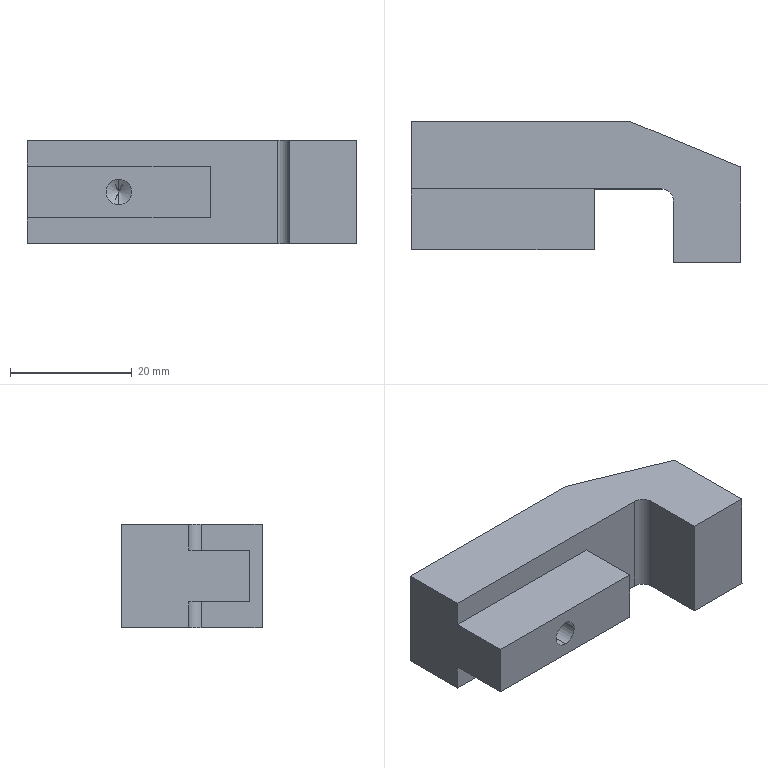Part | STEP file | PN_0002  Clamp_Default | 1 solid | 18 faces | box 54 x 23 x 17 mm | volume 13573 mm3 | plane 13 | cylinder 3 | cone 2 | commonest cylinder face diameters 4.2 x2 4 x1
STEP:
#1=CARTESIAN_POINT('',(0.,0.,0.));
#2=DIRECTION('',(0.,0.,1.));
#3=DIRECTION('',(1.,0.,0.));
#4=AXIS2_PLACEMENT_3D('',#1,#2,#3);
#5=CARTESIAN_POINT('',(15.,-7.,-2.1));
#6=VERTEX_POINT('',#5);
#7=CARTESIAN_POINT('',(15.,-21.,-2.1));
#8=VERTEX_POINT('',#7);
#9=CARTESIAN_POINT('',(15.,-21.,-2.1));
#10=DIRECTION('',(0.,-1.,0.));
#11=VECTOR('',#10,1.);
#12=LINE('',#9,#11);
#13=CARTESIAN_POINT('',(15.,-21.,0.));
#14=DIRECTION('',(0.,-1.,0.));
#15=DIRECTION('',(0.,0.,-1.));
#16=AXIS2_PLACEMENT_3D('',#13,#14,#15);
#17=CYLINDRICAL_SURFACE('',#16,2.1);
#18=CARTESIAN_POINT('',(6.283,0.));
#19=DIRECTION('',(0.,1.));
#20=VECTOR('',#19,1.);
#21=LINE('',#18,#20);
#22=(GEOMETRIC_REPRESENTATION_CONTEXT(2)PARAMETRIC_REPRESENTATION_CONTEXT()REPRESENTATION_CONTEXT('',''));
#23=DEFINITIONAL_REPRESENTATION('',(#21),#22);
#24=PCURVE('',#17,#23);
#25=CARTESIAN_POINT('',(15.,-21.,0.));
#26=DIRECTION('',(0.,-1.,0.));
#27=DIRECTION('',(0.,0.,-1.));
#28=AXIS2_PLACEMENT_3D('',#25,#26,#27);
#29=CYLINDRICAL_SURFACE('',#28,2.1);
#30=CARTESIAN_POINT('',(0.,0.));
#31=DIRECTION('',(0.,1.));
#32=VECTOR('',#31,1.);
#33=LINE('',#30,#32);
#34=(GEOMETRIC_REPRESENTATION_CONTEXT(2)PARAMETRIC_REPRESENTATION_CONTEXT()REPRESENTATION_CONTEXT('',''));
#35=DEFINITIONAL_REPRESENTATION('',(#33),#34);
#36=PCURVE('',#29,#35);
#37=SURFACE_CURVE('',#12,(#24,#36),.PCURVE_S1.);
#38=EDGE_CURVE('',#6,#8,#37,.T.);
#39=ORIENTED_EDGE('',*,*,#38,.T.);
#40=CARTESIAN_POINT('',(15.,-21.,2.1));
#41=VERTEX_POINT('',#40);
#42=CARTESIAN_POINT('',(15.,-21.,0.));
#43=DIRECTION('',(0.,-1.,0.));
#44=DIRECTION('',(0.,0.,-1.));
#45=AXIS2_PLACEMENT_3D('',#42,#43,#44);
#46=CIRCLE('',#45,2.1);
#47=CARTESIAN_POINT('',(0.,0.));
#48=DIRECTION('',(1.,0.));
#49=VECTOR('',#48,1.);
#50=LINE('',#47,#49);
#51=(GEOMETRIC_REPRESENTATION_CONTEXT(2)PARAMETRIC_REPRESENTATION_CONTEXT()REPRESENTATION_CONTEXT('',''));
#52=DEFINITIONAL_REPRESENTATION('',(#50),#51);
#53=PCURVE('',#17,#52);
#54=CARTESIAN_POINT('',(0.,-21.,0.));
#55=DIRECTION('',(0.,-1.,0.));
#56=DIRECTION('',(1.,0.,0.));
#57=AXIS2_PLACEMENT_3D('',#54,#55,#56);
#58=PLANE('',#57);
#59=CARTESIAN_POINT('',(15.,0.));
#60=DIRECTION('',(0.,-1.));
#61=AXIS2_PLACEMENT_2D('',#59,#60);
#62=CIRCLE('',#61,2.1);
#63=(GEOMETRIC_REPRESENTATION_CONTEXT(2)PARAMETRIC_REPRESENTATION_CONTEXT()REPRESENTATION_CONTEXT('',''));
#64=DEFINITIONAL_REPRESENTATION('',(#62),#63);
#65=PCURVE('',#58,#64);
#66=SURFACE_CURVE('',#46,(#53,#65),.PCURVE_S1.);
#67=EDGE_CURVE('',#41,#8,#66,.T.);
#68=ORIENTED_EDGE('',*,*,#67,.F.);
#69=CARTESIAN_POINT('',(15.,-7.,2.1));
#70=VERTEX_POINT('',#69);
#71=CARTESIAN_POINT('',(15.,-21.,2.1));
#72=DIRECTION('',(0.,-1.,0.));
#73=VECTOR('',#72,1.);
#74=LINE('',#71,#73);
#75=CARTESIAN_POINT('',(3.142,0.));
#76=DIRECTION('',(0.,1.));
#77=VECTOR('',#76,1.);
#78=LINE('',#75,#77);
#79=(GEOMETRIC_REPRESENTATION_CONTEXT(2)PARAMETRIC_REPRESENTATION_CONTEXT()REPRESENTATION_CONTEXT('',''));
#80=DEFINITIONAL_REPRESENTATION('',(#78),#79);
#81=PCURVE('',#17,#80);
#82=CARTESIAN_POINT('',(3.142,0.));
#83=DIRECTION('',(0.,1.));
#84=VECTOR('',#83,1.);
#85=LINE('',#82,#84);
#86=(GEOMETRIC_REPRESENTATION_CONTEXT(2)PARAMETRIC_REPRESENTATION_CONTEXT()REPRESENTATION_CONTEXT('',''));
#87=DEFINITIONAL_REPRESENTATION('',(#85),#86);
#88=PCURVE('',#29,#87);
#89=SURFACE_CURVE('',#74,(#81,#88),.PCURVE_S1.);
#90=EDGE_CURVE('',#70,#41,#89,.T.);
#91=ORIENTED_EDGE('',*,*,#90,.F.);
#92=CARTESIAN_POINT('',(15.,-7.,0.));
#93=DIRECTION('',(0.,-1.,0.));
#94=DIRECTION('',(0.,0.,-1.));
#95=AXIS2_PLACEMENT_3D('',#92,#93,#94);
#96=CIRCLE('',#95,2.1);
#97=CARTESIAN_POINT('',(0.,-14.));
#98=DIRECTION('',(1.,0.));
#99=VECTOR('',#98,1.);
#100=LINE('',#97,#99);
#101=(GEOMETRIC_REPRESENTATION_CONTEXT(2)PARAMETRIC_REPRESENTATION_CONTEXT()REPRESENTATION_CONTEXT('',''));
#102=DEFINITIONAL_REPRESENTATION('',(#100),#101);
#103=PCURVE('',#17,#102);
#104=CARTESIAN_POINT('',(15.,-7.,0.));
#105=DIRECTION('',(0.,-1.,0.));
#106=DIRECTION('',(0.,0.,-1.));
#107=AXIS2_PLACEMENT_3D('',#104,#105,#106);
#108=CONICAL_SURFACE('',#107,2.1,1.03);
#109=CARTESIAN_POINT('',(0.,0.));
#110=DIRECTION('',(1.,0.));
#111=VECTOR('',#110,1.);
#112=LINE('',#109,#111);
#113=(GEOMETRIC_REPRESENTATION_CONTEXT(2)PARAMETRIC_REPRESENTATION_CONTEXT()REPRESENTATION_CONTEXT('',''));
#114=DEFINITIONAL_REPRESENTATION('',(#112),#113);
#115=PCURVE('',#108,#114);
#116=SURFACE_CURVE('',#96,(#103,#115),.PCURVE_S1.);
#117=EDGE_CURVE('',#70,#6,#116,.T.);
#118=ORIENTED_EDGE('',*,*,#117,.T.);
#119=EDGE_LOOP('',(#39,#68,#91,#118));
#120=FACE_BOUND('',#119,.F.);
#121=ADVANCED_FACE('',(#120),#17,.F.);
#122=ORIENTED_EDGE('',*,*,#117,.F.);
#123=CARTESIAN_POINT('',(15.,-5.738,0.));
#124=VERTEX_POINT('',#123);
#125=CARTESIAN_POINT('',(15.,-7.,2.1));
#126=DIRECTION('',(0.,-0.515,0.8572));
#127=VECTOR('',#126,1.);
#128=LINE('',#125,#127);
#129=CARTESIAN_POINT('',(3.142,0.));
#130=DIRECTION('',(0.,1.));
#131=VECTOR('',#130,1.);
#132=LINE('',#129,#131);
#133=(GEOMETRIC_REPRESENTATION_CONTEXT(2)PARAMETRIC_REPRESENTATION_CONTEXT()REPRESENTATION_CONTEXT('',''));
#134=DEFINITIONAL_REPRESENTATION('',(#132),#133);
#135=PCURVE('',#108,#134);
#136=CARTESIAN_POINT('',(15.,-7.,0.));
#137=DIRECTION('',(0.,-1.,0.));
#138=DIRECTION('',(0.,0.,-1.));
#139=AXIS2_PLACEMENT_3D('',#136,#137,#138);
#140=CONICAL_SURFACE('',#139,2.1,1.03);
#141=CARTESIAN_POINT('',(3.142,0.));
#142=DIRECTION('',(0.,1.));
#143=VECTOR('',#142,1.);
#144=LINE('',#141,#143);
#145=(GEOMETRIC_REPRESENTATION_CONTEXT(2)PARAMETRIC_REPRESENTATION_CONTEXT()REPRESENTATION_CONTEXT('',''));
#146=DEFINITIONAL_REPRESENTATION('',(#144),#145);
#147=PCURVE('',#140,#146);
#148=SURFACE_CURVE('',#128,(#135,#147),.PCURVE_S1.);
#149=EDGE_CURVE('',#124,#70,#148,.T.);
#150=ORIENTED_EDGE('',*,*,#149,.F.);
#151=CARTESIAN_POINT('',(15.,-7.,-2.1));
#152=DIRECTION('',(0.,-0.515,-0.8572));
#153=VECTOR('',#152,1.);
#154=LINE('',#151,#153);
#155=CARTESIAN_POINT('',(6.283,0.));
#156=DIRECTION('',(0.,1.));
#157=VECTOR('',#156,1.);
#158=LINE('',#155,#157);
#159=(GEOMETRIC_REPRESENTATION_CONTEXT(2)PARAMETRIC_REPRESENTATION_CONTEXT()REPRESENTATION_CONTEXT('',''));
#160=DEFINITIONAL_REPRESENTATION('',(#158),#159);
#161=PCURVE('',#108,#160);
#162=CARTESIAN_POINT('',(0.,0.));
#163=DIRECTION('',(0.,1.));
#164=VECTOR('',#163,1.);
#165=LINE('',#162,#164);
#166=(GEOMETRIC_REPRESENTATION_CONTEXT(2)PARAMETRIC_REPRESENTATION_CONTEXT()REPRESENTATION_CONTEXT('',''));
#167=DEFINITIONAL_REPRESENTATION('',(#165),#166);
#168=PCURVE('',#140,#167);
#169=SURFACE_CURVE('',#154,(#161,#168),.PCURVE_S1.);
#170=EDGE_CURVE('',#124,#6,#169,.T.);
#171=ORIENTED_EDGE('',*,*,#170,.T.);
#172=EDGE_LOOP('',(#122,#150,#171));
#173=FACE_BOUND('',#172,.F.);
#174=ADVANCED_FACE('',(#173),#108,.F.);
#175=CARTESIAN_POINT('',(54.,-23.,-8.5));
#176=VERTEX_POINT('',#175);
#177=CARTESIAN_POINT('',(54.,-7.412,-8.5));
#178=VERTEX_POINT('',#177);
#179=CARTESIAN_POINT('',(54.,-15.,-8.5));
#180=DIRECTION('',(0.,1.,0.));
#181=VECTOR('',#180,1.);
#182=LINE('',#179,#181);
#183=CARTESIAN_POINT('',(54.,-15.,8.5));
#184=DIRECTION('',(-1.,0.,0.));
#185=DIRECTION('',(0.,0.,1.));
#186=AXIS2_PLACEMENT_3D('',#183,#184,#185);
#187=PLANE('',#186);
#188=CARTESIAN_POINT('',(-17.,0.));
#189=DIRECTION('',(0.,1.));
#190=VECTOR('',#189,1.);
#191=LINE('',#188,#190);
#192=(GEOMETRIC_REPRESENTATION_CONTEXT(2)PARAMETRIC_REPRESENTATION_CONTEXT()REPRESENTATION_CONTEXT('',''));
#193=DEFINITIONAL_REPRESENTATION('',(#191),#192);
#194=PCURVE('',#187,#193);
#195=CARTESIAN_POINT('',(0.,0.,-8.5));
#196=DIRECTION('',(0.,0.,1.));
#197=DIRECTION('',(1.,0.,0.));
#198=AXIS2_PLACEMENT_3D('',#195,#196,#197);
#199=PLANE('',#198);
#200=CARTESIAN_POINT('',(54.,-15.));
#201=DIRECTION('',(0.,1.));
#202=VECTOR('',#201,1.);
#203=LINE('',#200,#202);
#204=(GEOMETRIC_REPRESENTATION_CONTEXT(2)PARAMETRIC_REPRESENTATION_CONTEXT()REPRESENTATION_CONTEXT('',''));
#205=DEFINITIONAL_REPRESENTATION('',(#203),#204);
#206=PCURVE('',#199,#205);
#207=SURFACE_CURVE('',#182,(#194,#206),.PCURVE_S1.);
#208=EDGE_CURVE('',#176,#178,#207,.T.);
#209=ORIENTED_EDGE('',*,*,#208,.T.);
#210=CARTESIAN_POINT('',(54.,-7.412,8.5));
#211=VERTEX_POINT('',#210);
#212=CARTESIAN_POINT('',(54.,-7.412,8.5));
#213=DIRECTION('',(0.,0.,-1.));
#214=VECTOR('',#213,1.);
#215=LINE('',#212,#214);
#216=CARTESIAN_POINT('',(0.,7.588));
#217=DIRECTION('',(-1.,0.));
#218=VECTOR('',#217,1.);
#219=LINE('',#216,#218);
#220=(GEOMETRIC_REPRESENTATION_CONTEXT(2)PARAMETRIC_REPRESENTATION_CONTEXT()REPRESENTATION_CONTEXT('',''));
#221=DEFINITIONAL_REPRESENTATION('',(#219),#220);
#222=PCURVE('',#187,#221);
#223=CARTESIAN_POINT('',(54.,-7.412,8.5));
#224=DIRECTION('',(-0.3807,-0.9247,0.));
#225=DIRECTION('',(0.9247,-0.3807,0.));
#226=AXIS2_PLACEMENT_3D('',#223,#224,#225);
#227=PLANE('',#226);
#228=CARTESIAN_POINT('',(0.,0.));
#229=DIRECTION('',(0.,-1.));
#230=VECTOR('',#229,1.);
#231=LINE('',#228,#230);
#232=(GEOMETRIC_REPRESENTATION_CONTEXT(2)PARAMETRIC_REPRESENTATION_CONTEXT()REPRESENTATION_CONTEXT('',''));
#233=DEFINITIONAL_REPRESENTATION('',(#231),#232);
#234=PCURVE('',#227,#233);
#235=SURFACE_CURVE('',#215,(#222,#234),.PCURVE_S1.);
#236=EDGE_CURVE('',#211,#178,#235,.T.);
#237=ORIENTED_EDGE('',*,*,#236,.F.);
#238=CARTESIAN_POINT('',(54.,-23.,8.5));
#239=VERTEX_POINT('',#238);
#240=CARTESIAN_POINT('',(54.,-15.,8.5));
#241=DIRECTION('',(0.,1.,0.));
#242=VECTOR('',#241,1.);
#243=LINE('',#240,#242);
#244=CARTESIAN_POINT('',(0.,0.));
#245=DIRECTION('',(0.,1.));
#246=VECTOR('',#245,1.);
#247=LINE('',#244,#246);
#248=(GEOMETRIC_REPRESENTATION_CONTEXT(2)PARAMETRIC_REPRESENTATION_CONTEXT()REPRESENTATION_CONTEXT('',''));
#249=DEFINITIONAL_REPRESENTATION('',(#247),#248);
#250=PCURVE('',#187,#249);
#251=CARTESIAN_POINT('',(0.,0.,8.5));
#252=DIRECTION('',(0.,0.,1.));
#253=DIRECTION('',(1.,0.,0.));
#254=AXIS2_PLACEMENT_3D('',#251,#252,#253);
#255=PLANE('',#254);
#256=CARTESIAN_POINT('',(54.,-15.));
#257=DIRECTION('',(0.,1.));
#258=VECTOR('',#257,1.);
#259=LINE('',#256,#258);
#260=(GEOMETRIC_REPRESENTATION_CONTEXT(2)PARAMETRIC_REPRESENTATION_CONTEXT()REPRESENTATION_CONTEXT('',''));
#261=DEFINITIONAL_REPRESENTATION('',(#259),#260);
#262=PCURVE('',#255,#261);
#263=SURFACE_CURVE('',#243,(#250,#262),.PCURVE_S1.);
#264=EDGE_CURVE('',#239,#211,#263,.T.);
#265=ORIENTED_EDGE('',*,*,#264,.F.);
#266=CARTESIAN_POINT('',(54.,-23.,8.5));
#267=DIRECTION('',(0.,0.,1.));
#268=VECTOR('',#267,1.);
#269=LINE('',#266,#268);
#270=CARTESIAN_POINT('',(0.,-8.));
#271=DIRECTION('',(1.,0.));
#272=VECTOR('',#271,1.);
#273=LINE('',#270,#272);
#274=(GEOMETRIC_REPRESENTATION_CONTEXT(2)PARAMETRIC_REPRESENTATION_CONTEXT()REPRESENTATION_CONTEXT('',''));
#275=DEFINITIONAL_REPRESENTATION('',(#273),#274);
#276=PCURVE('',#187,#275);
#277=CARTESIAN_POINT('',(0.,-23.,0.));
#278=DIRECTION('',(0.,-1.,0.));
#279=DIRECTION('',(0.,0.,-1.));
#280=AXIS2_PLACEMENT_3D('',#277,#278,#279);
#281=PLANE('',#280);
#282=CARTESIAN_POINT('',(-8.5,54.));
#283=DIRECTION('',(-1.,0.));
#284=VECTOR('',#283,1.);
#285=LINE('',#282,#284);
#286=(GEOMETRIC_REPRESENTATION_CONTEXT(2)PARAMETRIC_REPRESENTATION_CONTEXT()REPRESENTATION_CONTEXT('',''));
#287=DEFINITIONAL_REPRESENTATION('',(#285),#286);
#288=PCURVE('',#281,#287);
#289=SURFACE_CURVE('',#269,(#276,#288),.PCURVE_S1.);
#290=EDGE_CURVE('',#176,#239,#289,.T.);
#291=ORIENTED_EDGE('',*,*,#290,.F.);
#292=EDGE_LOOP('',(#209,#237,#265,#291));
#293=FACE_BOUND('',#292,.T.);
#294=ADVANCED_FACE('',(#293),#187,.F.);
#295=CARTESIAN_POINT('',(36.,0.,-8.5));
#296=VERTEX_POINT('',#295);
#297=CARTESIAN_POINT('',(54.,-7.412,-8.5));
#298=DIRECTION('',(-0.9247,0.3807,0.));
#299=VECTOR('',#298,1.);
#300=LINE('',#297,#299);
#301=CARTESIAN_POINT('',(0.,-17.));
#302=DIRECTION('',(-1.,0.));
#303=VECTOR('',#302,1.);
#304=LINE('',#301,#303);
#305=(GEOMETRIC_REPRESENTATION_CONTEXT(2)PARAMETRIC_REPRESENTATION_CONTEXT()REPRESENTATION_CONTEXT('',''));
#306=DEFINITIONAL_REPRESENTATION('',(#304),#305);
#307=PCURVE('',#227,#306);
#308=CARTESIAN_POINT('',(54.,-7.412));
#309=DIRECTION('',(-0.9247,0.3807));
#310=VECTOR('',#309,1.);
#311=LINE('',#308,#310);
#312=(GEOMETRIC_REPRESENTATION_CONTEXT(2)PARAMETRIC_REPRESENTATION_CONTEXT()REPRESENTATION_CONTEXT('',''));
#313=DEFINITIONAL_REPRESENTATION('',(#311),#312);
#314=PCURVE('',#199,#313);
#315=SURFACE_CURVE('',#300,(#307,#314),.PCURVE_S1.);
#316=EDGE_CURVE('',#178,#296,#315,.T.);
#317=ORIENTED_EDGE('',*,*,#316,.T.);
#318=CARTESIAN_POINT('',(36.,0.,8.5));
#319=VERTEX_POINT('',#318);
#320=CARTESIAN_POINT('',(36.,0.,8.5));
#321=DIRECTION('',(0.,0.,-1.));
#322=VECTOR('',#321,1.);
#323=LINE('',#320,#322);
#324=CARTESIAN_POINT('',(-19.466,0.));
#325=DIRECTION('',(0.,-1.));
#326=VECTOR('',#325,1.);
#327=LINE('',#324,#326);
#328=(GEOMETRIC_REPRESENTATION_CONTEXT(2)PARAMETRIC_REPRESENTATION_CONTEXT()REPRESENTATION_CONTEXT('',''));
#329=DEFINITIONAL_REPRESENTATION('',(#327),#328);
#330=PCURVE('',#227,#329);
#331=CARTESIAN_POINT('',(36.,0.,8.5));
#332=DIRECTION('',(0.,-1.,0.));
#333=DIRECTION('',(1.,0.,0.));
#334=AXIS2_PLACEMENT_3D('',#331,#332,#333);
#335=PLANE('',#334);
#336=CARTESIAN_POINT('',(0.,0.));
#337=DIRECTION('',(0.,-1.));
#338=VECTOR('',#337,1.);
#339=LINE('',#336,#338);
#340=(GEOMETRIC_REPRESENTATION_CONTEXT(2)PARAMETRIC_REPRESENTATION_CONTEXT()REPRESENTATION_CONTEXT('',''));
#341=DEFINITIONAL_REPRESENTATION('',(#339),#340);
#342=PCURVE('',#335,#341);
#343=SURFACE_CURVE('',#323,(#330,#342),.PCURVE_S1.);
#344=EDGE_CURVE('',#319,#296,#343,.T.);
#345=ORIENTED_EDGE('',*,*,#344,.F.);
#346=CARTESIAN_POINT('',(54.,-7.412,8.5));
#347=DIRECTION('',(-0.9247,0.3807,0.));
#348=VECTOR('',#347,1.);
#349=LINE('',#346,#348);
#350=CARTESIAN_POINT('',(0.,0.));
#351=DIRECTION('',(-1.,0.));
#352=VECTOR('',#351,1.);
#353=LINE('',#350,#352);
#354=(GEOMETRIC_REPRESENTATION_CONTEXT(2)PARAMETRIC_REPRESENTATION_CONTEXT()REPRESENTATION_CONTEXT('',''));
#355=DEFINITIONAL_REPRESENTATION('',(#353),#354);
#356=PCURVE('',#227,#355);
#357=CARTESIAN_POINT('',(54.,-7.412));
#358=DIRECTION('',(-0.9247,0.3807));
#359=VECTOR('',#358,1.);
#360=LINE('',#357,#359);
#361=(GEOMETRIC_REPRESENTATION_CONTEXT(2)PARAMETRIC_REPRESENTATION_CONTEXT()REPRESENTATION_CONTEXT('',''));
#362=DEFINITIONAL_REPRESENTATION('',(#360),#361);
#363=PCURVE('',#255,#362);
#364=SURFACE_CURVE('',#349,(#356,#363),.PCURVE_S1.);
#365=EDGE_CURVE('',#211,#319,#364,.T.);
#366=ORIENTED_EDGE('',*,*,#365,.F.);
#367=ORIENTED_EDGE('',*,*,#236,.T.);
#368=EDGE_LOOP('',(#317,#345,#366,#367));
#369=FACE_BOUND('',#368,.T.);
#370=ADVANCED_FACE('',(#369),#227,.F.);
#371=CARTESIAN_POINT('',(0.,0.,-8.5));
#372=VERTEX_POINT('',#371);
#373=CARTESIAN_POINT('',(36.,0.,-8.5));
#374=DIRECTION('',(-1.,0.,0.));
#375=VECTOR('',#374,1.);
#376=LINE('',#373,#375);
#377=CARTESIAN_POINT('',(0.,-17.));
#378=DIRECTION('',(-1.,0.));
#379=VECTOR('',#378,1.);
#380=LINE('',#377,#379);
#381=(GEOMETRIC_REPRESENTATION_CONTEXT(2)PARAMETRIC_REPRESENTATION_CONTEXT()REPRESENTATION_CONTEXT('',''));
#382=DEFINITIONAL_REPRESENTATION('',(#380),#381);
#383=PCURVE('',#335,#382);
#384=CARTESIAN_POINT('',(36.,0.));
#385=DIRECTION('',(-1.,0.));
#386=VECTOR('',#385,1.);
#387=LINE('',#384,#386);
#388=(GEOMETRIC_REPRESENTATION_CONTEXT(2)PARAMETRIC_REPRESENTATION_CONTEXT()REPRESENTATION_CONTEXT('',''));
#389=DEFINITIONAL_REPRESENTATION('',(#387),#388);
#390=PCURVE('',#199,#389);
#391=SURFACE_CURVE('',#376,(#383,#390),.PCURVE_S1.);
#392=EDGE_CURVE('',#296,#372,#391,.T.);
#393=ORIENTED_EDGE('',*,*,#392,.T.);
#394=CARTESIAN_POINT('',(0.,0.,8.5));
#395=VERTEX_POINT('',#394);
#396=CARTESIAN_POINT('',(0.,0.,8.5));
#397=DIRECTION('',(0.,0.,-1.));
#398=VECTOR('',#397,1.);
#399=LINE('',#396,#398);
#400=CARTESIAN_POINT('',(-36.,0.));
#401=DIRECTION('',(0.,-1.));
#402=VECTOR('',#401,1.);
#403=LINE('',#400,#402);
#404=(GEOMETRIC_REPRESENTATION_CONTEXT(2)PARAMETRIC_REPRESENTATION_CONTEXT()REPRESENTATION_CONTEXT('',''));
#405=DEFINITIONAL_REPRESENTATION('',(#403),#404);
#406=PCURVE('',#335,#405);
#407=CARTESIAN_POINT('',(0.,0.,8.5));
#408=DIRECTION('',(1.,0.000000213,0.));
#409=DIRECTION('',(-0.000000213,1.,0.));
#410=AXIS2_PLACEMENT_3D('',#407,#408,#409);
#411=PLANE('',#410);
#412=CARTESIAN_POINT('',(0.,0.));
#413=DIRECTION('',(0.,-1.));
#414=VECTOR('',#413,1.);
#415=LINE('',#412,#414);
#416=(GEOMETRIC_REPRESENTATION_CONTEXT(2)PARAMETRIC_REPRESENTATION_CONTEXT()REPRESENTATION_CONTEXT('',''));
#417=DEFINITIONAL_REPRESENTATION('',(#415),#416);
#418=PCURVE('',#411,#417);
#419=SURFACE_CURVE('',#399,(#406,#418),.PCURVE_S1.);
#420=EDGE_CURVE('',#395,#372,#419,.T.);
#421=ORIENTED_EDGE('',*,*,#420,.F.);
#422=CARTESIAN_POINT('',(36.,0.,8.5));
#423=DIRECTION('',(-1.,0.,0.));
#424=VECTOR('',#423,1.);
#425=LINE('',#422,#424);
#426=CARTESIAN_POINT('',(0.,0.));
#427=DIRECTION('',(-1.,0.));
#428=VECTOR('',#427,1.);
#429=LINE('',#426,#428);
#430=(GEOMETRIC_REPRESENTATION_CONTEXT(2)PARAMETRIC_REPRESENTATION_CONTEXT()REPRESENTATION_CONTEXT('',''));
#431=DEFINITIONAL_REPRESENTATION('',(#429),#430);
#432=PCURVE('',#335,#431);
#433=CARTESIAN_POINT('',(36.,0.));
#434=DIRECTION('',(-1.,0.));
#435=VECTOR('',#434,1.);
#436=LINE('',#433,#435);
#437=(GEOMETRIC_REPRESENTATION_CONTEXT(2)PARAMETRIC_REPRESENTATION_CONTEXT()REPRESENTATION_CONTEXT('',''));
#438=DEFINITIONAL_REPRESENTATION('',(#436),#437);
#439=PCURVE('',#255,#438);
#440=SURFACE_CURVE('',#425,(#432,#439),.PCURVE_S1.);
#441=EDGE_CURVE('',#319,#395,#440,.T.);
#442=ORIENTED_EDGE('',*,*,#441,.F.);
#443=ORIENTED_EDGE('',*,*,#344,.T.);
#444=EDGE_LOOP('',(#393,#421,#442,#443));
#445=FACE_BOUND('',#444,.T.);
#446=ADVANCED_FACE('',(#445),#335,.F.);
#447=ORIENTED_EDGE('',*,*,#420,.F.);
#448=CARTESIAN_POINT('',(0.000003197,-11.,8.5));
#449=VERTEX_POINT('',#448);
#450=CARTESIAN_POINT('',(0.,0.,8.5));
#451=DIRECTION('',(0.000000213,-1.,0.));
#452=VECTOR('',#451,1.);
#453=LINE('',#450,#452);
#454=CARTESIAN_POINT('',(0.,0.));
#455=DIRECTION('',(-1.,0.));
#456=VECTOR('',#455,1.);
#457=LINE('',#454,#456);
#458=(GEOMETRIC_REPRESENTATION_CONTEXT(2)PARAMETRIC_REPRESENTATION_CONTEXT()REPRESENTATION_CONTEXT('',''));
#459=DEFINITIONAL_REPRESENTATION('',(#457),#458);
#460=PCURVE('',#411,#459);
#461=CARTESIAN_POINT('',(0.,0.));
#462=DIRECTION('',(0.000000213,-1.));
#463=VECTOR('',#462,1.);
#464=LINE('',#461,#463);
#465=(GEOMETRIC_REPRESENTATION_CONTEXT(2)PARAMETRIC_REPRESENTATION_CONTEXT()REPRESENTATION_CONTEXT('',''));
#466=DEFINITIONAL_REPRESENTATION('',(#464),#465);
#467=PCURVE('',#255,#466);
#468=SURFACE_CURVE('',#453,(#460,#467),.PCURVE_S1.);
#469=EDGE_CURVE('',#395,#449,#468,.T.);
#470=ORIENTED_EDGE('',*,*,#469,.T.);
#471=CARTESIAN_POINT('',(0.,-11.,4.25));
#472=VERTEX_POINT('',#471);
#473=CARTESIAN_POINT('',(0.000003197,-11.,8.5));
#474=DIRECTION('',(-0.000000752,0.,-1.));
#475=VECTOR('',#474,1.);
#476=LINE('',#473,#475);
#477=CARTESIAN_POINT('',(-11.,0.));
#478=DIRECTION('',(0.,-1.));
#479=VECTOR('',#478,1.);
#480=LINE('',#477,#479);
#481=(GEOMETRIC_REPRESENTATION_CONTEXT(2)PARAMETRIC_REPRESENTATION_CONTEXT()REPRESENTATION_CONTEXT('',''));
#482=DEFINITIONAL_REPRESENTATION('',(#480),#481);
#483=PCURVE('',#411,#482);
#484=CARTESIAN_POINT('',(30.,-11.,8.5));
#485=DIRECTION('',(0.,1.,0.));
#486=DIRECTION('',(-1.,0.,0.));
#487=AXIS2_PLACEMENT_3D('',#484,#485,#486);
#488=PLANE('',#487);
#489=CARTESIAN_POINT('',(30.,0.));
#490=DIRECTION('',(0.000000752,-1.));
#491=VECTOR('',#490,1.);
#492=LINE('',#489,#491);
#493=(GEOMETRIC_REPRESENTATION_CONTEXT(2)PARAMETRIC_REPRESENTATION_CONTEXT()REPRESENTATION_CONTEXT('',''));
#494=DEFINITIONAL_REPRESENTATION('',(#492),#493);
#495=PCURVE('',#488,#494);
#496=SURFACE_CURVE('',#476,(#483,#495),.PCURVE_S1.);
#497=EDGE_CURVE('',#449,#472,#496,.T.);
#498=ORIENTED_EDGE('',*,*,#497,.T.);
#499=CARTESIAN_POINT('',(0.,-21.,4.25));
#500=VERTEX_POINT('',#499);
#501=CARTESIAN_POINT('',(0.,23.989,4.25));
#502=DIRECTION('',(0.,-1.,0.));
#503=VECTOR('',#502,1.);
#504=LINE('',#501,#503);
#505=CARTESIAN_POINT('',(23.989,-4.25));
#506=DIRECTION('',(-1.,0.));
#507=VECTOR('',#506,1.);
#508=LINE('',#505,#507);
#509=(GEOMETRIC_REPRESENTATION_CONTEXT(2)PARAMETRIC_REPRESENTATION_CONTEXT()REPRESENTATION_CONTEXT('',''));
#510=DEFINITIONAL_REPRESENTATION('',(#508),#509);
#511=PCURVE('',#411,#510);
#512=CARTESIAN_POINT('',(0.,23.989,4.25));
#513=DIRECTION('',(0.,0.,-1.));
#514=DIRECTION('',(-1.,0.,0.));
#515=AXIS2_PLACEMENT_3D('',#512,#513,#514);
#516=PLANE('',#515);
#517=CARTESIAN_POINT('',(0.,0.));
#518=DIRECTION('',(0.,-1.));
#519=VECTOR('',#518,1.);
#520=LINE('',#517,#519);
#521=(GEOMETRIC_REPRESENTATION_CONTEXT(2)PARAMETRIC_REPRESENTATION_CONTEXT()REPRESENTATION_CONTEXT('',''));
#522=DEFINITIONAL_REPRESENTATION('',(#520),#521);
#523=PCURVE('',#516,#522);
#524=SURFACE_CURVE('',#504,(#511,#523),.PCURVE_S1.);
#525=EDGE_CURVE('',#472,#500,#524,.T.);
#526=ORIENTED_EDGE('',*,*,#525,.T.);
#527=CARTESIAN_POINT('',(0.,-21.,-4.25));
#528=VERTEX_POINT('',#527);
#529=CARTESIAN_POINT('',(0.,-21.,4.25));
#530=DIRECTION('',(0.,0.,-1.));
#531=VECTOR('',#530,1.);
#532=LINE('',#529,#531);
#533=CARTESIAN_POINT('',(-21.,-4.25));
#534=DIRECTION('',(0.,-1.));
#535=VECTOR('',#534,1.);
#536=LINE('',#533,#535);
#537=(GEOMETRIC_REPRESENTATION_CONTEXT(2)PARAMETRIC_REPRESENTATION_CONTEXT()REPRESENTATION_CONTEXT('',''));
#538=DEFINITIONAL_REPRESENTATION('',(#536),#537);
#539=PCURVE('',#411,#538);
#540=CARTESIAN_POINT('',(0.,4.25));
#541=DIRECTION('',(0.,-1.));
#542=VECTOR('',#541,1.);
#543=LINE('',#540,#542);
#544=(GEOMETRIC_REPRESENTATION_CONTEXT(2)PARAMETRIC_REPRESENTATION_CONTEXT()REPRESENTATION_CONTEXT('',''));
#545=DEFINITIONAL_REPRESENTATION('',(#543),#544);
#546=PCURVE('',#58,#545);
#547=SURFACE_CURVE('',#532,(#539,#546),.PCURVE_S1.);
#548=EDGE_CURVE('',#500,#528,#547,.T.);
#549=ORIENTED_EDGE('',*,*,#548,.T.);
#550=CARTESIAN_POINT('',(0.,-11.,-4.25));
#551=VERTEX_POINT('',#550);
#552=CARTESIAN_POINT('',(0.,23.989,-4.25));
#553=DIRECTION('',(0.,-1.,0.));
#554=VECTOR('',#553,1.);
#555=LINE('',#552,#554);
#556=CARTESIAN_POINT('',(23.989,-12.75));
#557=DIRECTION('',(-1.,0.));
#558=VECTOR('',#557,1.);
#559=LINE('',#556,#558);
#560=(GEOMETRIC_REPRESENTATION_CONTEXT(2)PARAMETRIC_REPRESENTATION_CONTEXT()REPRESENTATION_CONTEXT('',''));
#561=DEFINITIONAL_REPRESENTATION('',(#559),#560);
#562=PCURVE('',#411,#561);
#563=CARTESIAN_POINT('',(0.,23.989,-4.25));
#564=DIRECTION('',(0.,0.,1.));
#565=DIRECTION('',(1.,0.,0.));
#566=AXIS2_PLACEMENT_3D('',#563,#564,#565);
#567=PLANE('',#566);
#568=CARTESIAN_POINT('',(0.,0.));
#569=DIRECTION('',(0.,-1.));
#570=VECTOR('',#569,1.);
#571=LINE('',#568,#570);
#572=(GEOMETRIC_REPRESENTATION_CONTEXT(2)PARAMETRIC_REPRESENTATION_CONTEXT()REPRESENTATION_CONTEXT('',''));
#573=DEFINITIONAL_REPRESENTATION('',(#571),#572);
#574=PCURVE('',#567,#573);
#575=SURFACE_CURVE('',#555,(#562,#574),.PCURVE_S1.);
#576=EDGE_CURVE('',#551,#528,#575,.T.);
#577=ORIENTED_EDGE('',*,*,#576,.F.);
#578=CARTESIAN_POINT('',(0.000002344,-11.,-8.5));
#579=VERTEX_POINT('',#578);
#580=CARTESIAN_POINT('',(0.000003197,-11.,-8.5));
#581=DIRECTION('',(0.000000752,0.,-1.));
#582=VECTOR('',#581,1.);
#583=LINE('',#580,#582);
#584=CARTESIAN_POINT('',(-11.,-17.));
#585=DIRECTION('',(0.,-1.));
#586=VECTOR('',#585,1.);
#587=LINE('',#584,#586);
#588=(GEOMETRIC_REPRESENTATION_CONTEXT(2)PARAMETRIC_REPRESENTATION_CONTEXT()REPRESENTATION_CONTEXT('',''));
#589=DEFINITIONAL_REPRESENTATION('',(#587),#588);
#590=PCURVE('',#411,#589);
#591=CARTESIAN_POINT('',(30.,-17.));
#592=DIRECTION('',(-0.000000752,-1.));
#593=VECTOR('',#592,1.);
#594=LINE('',#591,#593);
#595=(GEOMETRIC_REPRESENTATION_CONTEXT(2)PARAMETRIC_REPRESENTATION_CONTEXT()REPRESENTATION_CONTEXT('',''));
#596=DEFINITIONAL_REPRESENTATION('',(#594),#595);
#597=PCURVE('',#488,#596);
#598=SURFACE_CURVE('',#583,(#590,#597),.PCURVE_S1.);
#599=EDGE_CURVE('',#551,#579,#598,.T.);
#600=ORIENTED_EDGE('',*,*,#599,.T.);
#601=CARTESIAN_POINT('',(0.,0.,-8.5));
#602=DIRECTION('',(0.000000213,-1.,0.));
#603=VECTOR('',#602,1.);
#604=LINE('',#601,#603);
#605=CARTESIAN_POINT('',(0.,-17.));
#606=DIRECTION('',(-1.,0.));
#607=VECTOR('',#606,1.);
#608=LINE('',#605,#607);
#609=(GEOMETRIC_REPRESENTATION_CONTEXT(2)PARAMETRIC_REPRESENTATION_CONTEXT()REPRESENTATION_CONTEXT('',''));
#610=DEFINITIONAL_REPRESENTATION('',(#608),#609);
#611=PCURVE('',#411,#610);
#612=CARTESIAN_POINT('',(0.,0.));
#613=DIRECTION('',(0.000000213,-1.));
#614=VECTOR('',#613,1.);
#615=LINE('',#612,#614);
#616=(GEOMETRIC_REPRESENTATION_CONTEXT(2)PARAMETRIC_REPRESENTATION_CONTEXT()REPRESENTATION_CONTEXT('',''));
#617=DEFINITIONAL_REPRESENTATION('',(#615),#616);
#618=PCURVE('',#199,#617);
#619=SURFACE_CURVE('',#604,(#611,#618),.PCURVE_S1.);
#620=EDGE_CURVE('',#372,#579,#619,.T.);
#621=ORIENTED_EDGE('',*,*,#620,.F.);
#622=EDGE_LOOP('',(#447,#470,#498,#526,#549,#577,#600,#621));
#623=FACE_BOUND('',#622,.F.);
#624=ADVANCED_FACE('',(#623),#411,.F.);
#625=CARTESIAN_POINT('',(30.,-11.,4.25));
#626=VERTEX_POINT('',#625);
#627=CARTESIAN_POINT('',(30.,-21.,4.25));
#628=VERTEX_POINT('',#627);
#629=CARTESIAN_POINT('',(30.,-15.,4.25));
#630=DIRECTION('',(0.,-1.,0.));
#631=VECTOR('',#630,1.);
#632=LINE('',#629,#631);
#633=CARTESIAN_POINT('',(30.,-15.,8.5));
#634=DIRECTION('',(-1.,0.,0.));
#635=DIRECTION('',(0.,0.,1.));
#636=AXIS2_PLACEMENT_3D('',#633,#634,#635);
#637=PLANE('',#636);
#638=CARTESIAN_POINT('',(-4.25,0.));
#639=DIRECTION('',(0.,-1.));
#640=VECTOR('',#639,1.);
#641=LINE('',#638,#640);
#642=(GEOMETRIC_REPRESENTATION_CONTEXT(2)PARAMETRIC_REPRESENTATION_CONTEXT()REPRESENTATION_CONTEXT('',''));
#643=DEFINITIONAL_REPRESENTATION('',(#641),#642);
#644=PCURVE('',#637,#643);
#645=CARTESIAN_POINT('',(-30.,-38.989));
#646=DIRECTION('',(0.,-1.));
#647=VECTOR('',#646,1.);
#648=LINE('',#645,#647);
#649=(GEOMETRIC_REPRESENTATION_CONTEXT(2)PARAMETRIC_REPRESENTATION_CONTEXT()REPRESENTATION_CONTEXT('',''));
#650=DEFINITIONAL_REPRESENTATION('',(#648),#649);
#651=PCURVE('',#516,#650);
#652=SURFACE_CURVE('',#632,(#644,#651),.PCURVE_S1.);
#653=EDGE_CURVE('',#626,#628,#652,.T.);
#654=ORIENTED_EDGE('',*,*,#653,.T.);
#655=CARTESIAN_POINT('',(30.,-21.,-4.25));
#656=VERTEX_POINT('',#655);
#657=CARTESIAN_POINT('',(30.,-21.,-4.25));
#658=DIRECTION('',(0.,0.,1.));
#659=VECTOR('',#658,1.);
#660=LINE('',#657,#659);
#661=CARTESIAN_POINT('',(-12.75,-6.));
#662=DIRECTION('',(1.,0.));
#663=VECTOR('',#662,1.);
#664=LINE('',#661,#663);
#665=(GEOMETRIC_REPRESENTATION_CONTEXT(2)PARAMETRIC_REPRESENTATION_CONTEXT()REPRESENTATION_CONTEXT('',''));
#666=DEFINITIONAL_REPRESENTATION('',(#664),#665);
#667=PCURVE('',#637,#666);
#668=CARTESIAN_POINT('',(30.,-4.25));
#669=DIRECTION('',(0.,1.));
#670=VECTOR('',#669,1.);
#671=LINE('',#668,#670);
#672=(GEOMETRIC_REPRESENTATION_CONTEXT(2)PARAMETRIC_REPRESENTATION_CONTEXT()REPRESENTATION_CONTEXT('',''));
#673=DEFINITIONAL_REPRESENTATION('',(#671),#672);
#674=PCURVE('',#58,#673);
#675=SURFACE_CURVE('',#660,(#667,#674),.PCURVE_S1.);
#676=EDGE_CURVE('',#656,#628,#675,.T.);
#677=ORIENTED_EDGE('',*,*,#676,.F.);
#678=CARTESIAN_POINT('',(30.,-11.,-4.25));
#679=VERTEX_POINT('',#678);
#680=CARTESIAN_POINT('',(30.,-15.,-4.25));
#681=DIRECTION('',(0.,1.,0.));
#682=VECTOR('',#681,1.);
#683=LINE('',#680,#682);
#684=CARTESIAN_POINT('',(-12.75,0.));
#685=DIRECTION('',(0.,1.));
#686=VECTOR('',#685,1.);
#687=LINE('',#684,#686);
#688=(GEOMETRIC_REPRESENTATION_CONTEXT(2)PARAMETRIC_REPRESENTATION_CONTEXT()REPRESENTATION_CONTEXT('',''));
#689=DEFINITIONAL_REPRESENTATION('',(#687),#688);
#690=PCURVE('',#637,#689);
#691=CARTESIAN_POINT('',(30.,-38.989));
#692=DIRECTION('',(0.,1.));
#693=VECTOR('',#692,1.);
#694=LINE('',#691,#693);
#695=(GEOMETRIC_REPRESENTATION_CONTEXT(2)PARAMETRIC_REPRESENTATION_CONTEXT()REPRESENTATION_CONTEXT('',''));
#696=DEFINITIONAL_REPRESENTATION('',(#694),#695);
#697=PCURVE('',#567,#696);
#698=SURFACE_CURVE('',#683,(#690,#697),.PCURVE_S1.);
#699=EDGE_CURVE('',#656,#679,#698,.T.);
#700=ORIENTED_EDGE('',*,*,#699,.T.);
#701=CARTESIAN_POINT('',(30.,-11.,8.5));
#702=DIRECTION('',(0.,0.,-1.));
#703=VECTOR('',#702,1.);
#704=LINE('',#701,#703);
#705=CARTESIAN_POINT('',(0.,4.));
#706=DIRECTION('',(-1.,0.));
#707=VECTOR('',#706,1.);
#708=LINE('',#705,#707);
#709=(GEOMETRIC_REPRESENTATION_CONTEXT(2)PARAMETRIC_REPRESENTATION_CONTEXT()REPRESENTATION_CONTEXT('',''));
#710=DEFINITIONAL_REPRESENTATION('',(#708),#709);
#711=PCURVE('',#637,#710);
#712=CARTESIAN_POINT('',(0.,0.));
#713=DIRECTION('',(0.,-1.));
#714=VECTOR('',#713,1.);
#715=LINE('',#712,#714);
#716=(GEOMETRIC_REPRESENTATION_CONTEXT(2)PARAMETRIC_REPRESENTATION_CONTEXT()REPRESENTATION_CONTEXT('',''));
#717=DEFINITIONAL_REPRESENTATION('',(#715),#716);
#718=PCURVE('',#488,#717);
#719=SURFACE_CURVE('',#704,(#711,#718),.PCURVE_S1.);
#720=EDGE_CURVE('',#626,#679,#719,.T.);
#721=ORIENTED_EDGE('',*,*,#720,.F.);
#722=EDGE_LOOP('',(#654,#677,#700,#721));
#723=FACE_BOUND('',#722,.T.);
#724=ADVANCED_FACE('',(#723),#637,.F.);
#725=CARTESIAN_POINT('',(41.,-11.,-8.5));
#726=VERTEX_POINT('',#725);
#727=CARTESIAN_POINT('',(30.,-11.,-8.5));
#728=DIRECTION('',(1.,0.,0.));
#729=VECTOR('',#728,1.);
#730=LINE('',#727,#729);
#731=CARTESIAN_POINT('',(0.,-17.));
#732=DIRECTION('',(-1.,0.));
#733=VECTOR('',#732,1.);
#734=LINE('',#731,#733);
#735=(GEOMETRIC_REPRESENTATION_CONTEXT(2)PARAMETRIC_REPRESENTATION_CONTEXT()REPRESENTATION_CONTEXT('',''));
#736=DEFINITIONAL_REPRESENTATION('',(#734),#735);
#737=PCURVE('',#488,#736);
#738=CARTESIAN_POINT('',(30.,-11.));
#739=DIRECTION('',(1.,0.));
#740=VECTOR('',#739,1.);
#741=LINE('',#738,#740);
#742=(GEOMETRIC_REPRESENTATION_CONTEXT(2)PARAMETRIC_REPRESENTATION_CONTEXT()REPRESENTATION_CONTEXT('',''));
#743=DEFINITIONAL_REPRESENTATION('',(#741),#742);
#744=PCURVE('',#199,#743);
#745=SURFACE_CURVE('',#730,(#737,#744),.PCURVE_S1.);
#746=EDGE_CURVE('',#579,#726,#745,.T.);
#747=ORIENTED_EDGE('',*,*,#746,.T.);
#748=CARTESIAN_POINT('',(41.,-11.,8.5));
#749=VERTEX_POINT('',#748);
#750=CARTESIAN_POINT('',(41.,-11.,8.5));
#751=DIRECTION('',(0.,0.,1.));
#752=VECTOR('',#751,1.);
#753=LINE('',#750,#752);
#754=CARTESIAN_POINT('',(-11.,0.));
#755=DIRECTION('',(0.,1.));
#756=VECTOR('',#755,1.);
#757=LINE('',#754,#756);
#758=(GEOMETRIC_REPRESENTATION_CONTEXT(2)PARAMETRIC_REPRESENTATION_CONTEXT()REPRESENTATION_CONTEXT('',''));
#759=DEFINITIONAL_REPRESENTATION('',(#757),#758);
#760=PCURVE('',#488,#759);
#761=CARTESIAN_POINT('',(41.,-13.,8.5));
#762=DIRECTION('',(0.,0.,1.));
#763=DIRECTION('',(1.,0.,0.));
#764=AXIS2_PLACEMENT_3D('',#761,#762,#763);
#765=CYLINDRICAL_SURFACE('',#764,2.);
#766=CARTESIAN_POINT('',(1.571,0.));
#767=DIRECTION('',(0.,1.));
#768=VECTOR('',#767,1.);
#769=LINE('',#766,#768);
#770=(GEOMETRIC_REPRESENTATION_CONTEXT(2)PARAMETRIC_REPRESENTATION_CONTEXT()REPRESENTATION_CONTEXT('',''));
#771=DEFINITIONAL_REPRESENTATION('',(#769),#770);
#772=PCURVE('',#765,#771);
#773=SURFACE_CURVE('',#753,(#760,#772),.PCURVE_S1.);
#774=EDGE_CURVE('',#726,#749,#773,.T.);
#775=ORIENTED_EDGE('',*,*,#774,.T.);
#776=CARTESIAN_POINT('',(30.,-11.,8.5));
#777=DIRECTION('',(1.,0.,0.));
#778=VECTOR('',#777,1.);
#779=LINE('',#776,#778);
#780=CARTESIAN_POINT('',(0.,0.));
#781=DIRECTION('',(-1.,0.));
#782=VECTOR('',#781,1.);
#783=LINE('',#780,#782);
#784=(GEOMETRIC_REPRESENTATION_CONTEXT(2)PARAMETRIC_REPRESENTATION_CONTEXT()REPRESENTATION_CONTEXT('',''));
#785=DEFINITIONAL_REPRESENTATION('',(#783),#784);
#786=PCURVE('',#488,#785);
#787=CARTESIAN_POINT('',(30.,-11.));
#788=DIRECTION('',(1.,0.));
#789=VECTOR('',#788,1.);
#790=LINE('',#787,#789);
#791=(GEOMETRIC_REPRESENTATION_CONTEXT(2)PARAMETRIC_REPRESENTATION_CONTEXT()REPRESENTATION_CONTEXT('',''));
#792=DEFINITIONAL_REPRESENTATION('',(#790),#791);
#793=PCURVE('',#255,#792);
#794=SURFACE_CURVE('',#779,(#786,#793),.PCURVE_S1.);
#795=EDGE_CURVE('',#449,#749,#794,.T.);
#796=ORIENTED_EDGE('',*,*,#795,.F.);
#797=ORIENTED_EDGE('',*,*,#497,.T.);
#798=CARTESIAN_POINT('',(0.,-11.,4.25));
#799=DIRECTION('',(1.,0.,0.));
#800=VECTOR('',#799,1.);
#801=LINE('',#798,#800);
#802=CARTESIAN_POINT('',(30.,-4.25));
#803=DIRECTION('',(-1.,0.));
#804=VECTOR('',#803,1.);
#805=LINE('',#802,#804);
#806=(GEOMETRIC_REPRESENTATION_CONTEXT(2)PARAMETRIC_REPRESENTATION_CONTEXT()REPRESENTATION_CONTEXT('',''));
#807=DEFINITIONAL_REPRESENTATION('',(#805),#806);
#808=PCURVE('',#488,#807);
#809=CARTESIAN_POINT('',(0.,-34.989));
#810=DIRECTION('',(-1.,0.));
#811=VECTOR('',#810,1.);
#812=LINE('',#809,#811);
#813=(GEOMETRIC_REPRESENTATION_CONTEXT(2)PARAMETRIC_REPRESENTATION_CONTEXT()REPRESENTATION_CONTEXT('',''));
#814=DEFINITIONAL_REPRESENTATION('',(#812),#813);
#815=PCURVE('',#516,#814);
#816=SURFACE_CURVE('',#801,(#808,#815),.PCURVE_S1.);
#817=EDGE_CURVE('',#472,#626,#816,.T.);
#818=ORIENTED_EDGE('',*,*,#817,.T.);
#819=ORIENTED_EDGE('',*,*,#720,.T.);
#820=CARTESIAN_POINT('',(0.,-11.,-4.25));
#821=DIRECTION('',(-1.,0.,0.));
#822=VECTOR('',#821,1.);
#823=LINE('',#820,#822);
#824=CARTESIAN_POINT('',(30.,-12.75));
#825=DIRECTION('',(1.,0.));
#826=VECTOR('',#825,1.);
#827=LINE('',#824,#826);
#828=(GEOMETRIC_REPRESENTATION_CONTEXT(2)PARAMETRIC_REPRESENTATION_CONTEXT()REPRESENTATION_CONTEXT('',''));
#829=DEFINITIONAL_REPRESENTATION('',(#827),#828);
#830=PCURVE('',#488,#829);
#831=CARTESIAN_POINT('',(0.,-34.989));
#832=DIRECTION('',(-1.,0.));
#833=VECTOR('',#832,1.);
#834=LINE('',#831,#833);
#835=(GEOMETRIC_REPRESENTATION_CONTEXT(2)PARAMETRIC_REPRESENTATION_CONTEXT()REPRESENTATION_CONTEXT('',''));
#836=DEFINITIONAL_REPRESENTATION('',(#834),#835);
#837=PCURVE('',#567,#836);
#838=SURFACE_CURVE('',#823,(#830,#837),.PCURVE_S1.);
#839=EDGE_CURVE('',#679,#551,#838,.T.);
#840=ORIENTED_EDGE('',*,*,#839,.T.);
#841=ORIENTED_EDGE('',*,*,#599,.T.);
#842=EDGE_LOOP('',(#747,#775,#796,#797,#818,#819,#840,#841));
#843=FACE_BOUND('',#842,.T.);
#844=ADVANCED_FACE('',(#843),#488,.F.);
#845=CARTESIAN_POINT('',(43.,-13.,8.5));
#846=VERTEX_POINT('',#845);
#847=CARTESIAN_POINT('',(43.,-23.,8.5));
#848=VERTEX_POINT('',#847);
#849=CARTESIAN_POINT('',(43.,-11.,8.5));
#850=DIRECTION('',(0.,-1.,0.));
#851=VECTOR('',#850,1.);
#852=LINE('',#849,#851);
#853=CARTESIAN_POINT('',(43.,-11.,8.5));
#854=DIRECTION('',(1.,0.,0.));
#855=DIRECTION('',(0.,0.,-1.));
#856=AXIS2_PLACEMENT_3D('',#853,#854,#855);
#857=PLANE('',#856);
#858=CARTESIAN_POINT('',(0.,0.));
#859=DIRECTION('',(0.,-1.));
#860=VECTOR('',#859,1.);
#861=LINE('',#858,#860);
#862=(GEOMETRIC_REPRESENTATION_CONTEXT(2)PARAMETRIC_REPRESENTATION_CONTEXT()REPRESENTATION_CONTEXT('',''));
#863=DEFINITIONAL_REPRESENTATION('',(#861),#862);
#864=PCURVE('',#857,#863);
#865=CARTESIAN_POINT('',(43.,-11.));
#866=DIRECTION('',(0.,-1.));
#867=VECTOR('',#866,1.);
#868=LINE('',#865,#867);
#869=(GEOMETRIC_REPRESENTATION_CONTEXT(2)PARAMETRIC_REPRESENTATION_CONTEXT()REPRESENTATION_CONTEXT('',''));
#870=DEFINITIONAL_REPRESENTATION('',(#868),#869);
#871=PCURVE('',#255,#870);
#872=SURFACE_CURVE('',#852,(#864,#871),.PCURVE_S1.);
#873=EDGE_CURVE('',#846,#848,#872,.T.);
#874=ORIENTED_EDGE('',*,*,#873,.F.);
#875=CARTESIAN_POINT('',(43.,-13.,-8.5));
#876=VERTEX_POINT('',#875);
#877=CARTESIAN_POINT('',(43.,-13.,-8.5));
#878=DIRECTION('',(0.,0.,-1.));
#879=VECTOR('',#878,1.);
#880=LINE('',#877,#879);
#881=CARTESIAN_POINT('',(17.,-2.));
#882=DIRECTION('',(1.,0.));
#883=VECTOR('',#882,1.);
#884=LINE('',#881,#883);
#885=(GEOMETRIC_REPRESENTATION_CONTEXT(2)PARAMETRIC_REPRESENTATION_CONTEXT()REPRESENTATION_CONTEXT('',''));
#886=DEFINITIONAL_REPRESENTATION('',(#884),#885);
#887=PCURVE('',#857,#886);
#888=CARTESIAN_POINT('',(0.,-17.));
#889=DIRECTION('',(0.,-1.));
#890=VECTOR('',#889,1.);
#891=LINE('',#888,#890);
#892=(GEOMETRIC_REPRESENTATION_CONTEXT(2)PARAMETRIC_REPRESENTATION_CONTEXT()REPRESENTATION_CONTEXT('',''));
#893=DEFINITIONAL_REPRESENTATION('',(#891),#892);
#894=PCURVE('',#765,#893);
#895=SURFACE_CURVE('',#880,(#887,#894),.PCURVE_S1.);
#896=EDGE_CURVE('',#846,#876,#895,.T.);
#897=ORIENTED_EDGE('',*,*,#896,.T.);
#898=CARTESIAN_POINT('',(43.,-23.,-8.5));
#899=VERTEX_POINT('',#898);
#900=CARTESIAN_POINT('',(43.,-11.,-8.5));
#901=DIRECTION('',(0.,-1.,0.));
#902=VECTOR('',#901,1.);
#903=LINE('',#900,#902);
#904=CARTESIAN_POINT('',(17.,0.));
#905=DIRECTION('',(0.,-1.));
#906=VECTOR('',#905,1.);
#907=LINE('',#904,#906);
#908=(GEOMETRIC_REPRESENTATION_CONTEXT(2)PARAMETRIC_REPRESENTATION_CONTEXT()REPRESENTATION_CONTEXT('',''));
#909=DEFINITIONAL_REPRESENTATION('',(#907),#908);
#910=PCURVE('',#857,#909);
#911=CARTESIAN_POINT('',(43.,-11.));
#912=DIRECTION('',(0.,-1.));
#913=VECTOR('',#912,1.);
#914=LINE('',#911,#913);
#915=(GEOMETRIC_REPRESENTATION_CONTEXT(2)PARAMETRIC_REPRESENTATION_CONTEXT()REPRESENTATION_CONTEXT('',''));
#916=DEFINITIONAL_REPRESENTATION('',(#914),#915);
#917=PCURVE('',#199,#916);
#918=SURFACE_CURVE('',#903,(#910,#917),.PCURVE_S1.);
#919=EDGE_CURVE('',#876,#899,#918,.T.);
#920=ORIENTED_EDGE('',*,*,#919,.T.);
#921=CARTESIAN_POINT('',(43.,-23.,8.5));
#922=DIRECTION('',(0.,0.,-1.));
#923=VECTOR('',#922,1.);
#924=LINE('',#921,#923);
#925=CARTESIAN_POINT('',(0.,-12.));
#926=DIRECTION('',(1.,0.));
#927=VECTOR('',#926,1.);
#928=LINE('',#925,#927);
#929=(GEOMETRIC_REPRESENTATION_CONTEXT(2)PARAMETRIC_REPRESENTATION_CONTEXT()REPRESENTATION_CONTEXT('',''));
#930=DEFINITIONAL_REPRESENTATION('',(#928),#929);
#931=PCURVE('',#857,#930);
#932=CARTESIAN_POINT('',(-8.5,43.));
#933=DIRECTION('',(1.,0.));
#934=VECTOR('',#933,1.);
#935=LINE('',#932,#934);
#936=(GEOMETRIC_REPRESENTATION_CONTEXT(2)PARAMETRIC_REPRESENTATION_CONTEXT()REPRESENTATION_CONTEXT('',''));
#937=DEFINITIONAL_REPRESENTATION('',(#935),#936);
#938=PCURVE('',#281,#937);
#939=SURFACE_CURVE('',#924,(#931,#938),.PCURVE_S1.);
#940=EDGE_CURVE('',#848,#899,#939,.T.);
#941=ORIENTED_EDGE('',*,*,#940,.F.);
#942=EDGE_LOOP('',(#874,#897,#920,#941));
#943=FACE_BOUND('',#942,.T.);
#944=ADVANCED_FACE('',(#943),#857,.F.);
#945=ORIENTED_EDGE('',*,*,#469,.T.);
#946=ORIENTED_EDGE('',*,*,#795,.T.);
#947=CARTESIAN_POINT('',(41.,-13.,8.5));
#948=DIRECTION('',(0.,0.,-1.));
#949=DIRECTION('',(1.,0.,0.));
#950=AXIS2_PLACEMENT_3D('',#947,#948,#949);
#951=CIRCLE('',#950,2.);
#952=CARTESIAN_POINT('',(43.,-13.));
#953=CARTESIAN_POINT('',(43.,-16.464));
#954=CARTESIAN_POINT('',(40.,-14.732));
#955=CARTESIAN_POINT('',(37.,-13.));
#956=CARTESIAN_POINT('',(40.,-11.268));
#957=CARTESIAN_POINT('',(43.,-9.536));
#958=CARTESIAN_POINT('',(43.,-13.));
#959=(BOUNDED_CURVE()B_SPLINE_CURVE(2,(#952,#953,#954,#955,#956,#957,#958),.UNSPECIFIED.,.T.,.F.)B_SPLINE_CURVE_WITH_KNOTS((1,2,2,2,2,1),(-2.094,0.,2.094,4.189,6.283,8.378),.UNSPECIFIED.)CURVE()GEOMETRIC_REPRESENTATION_ITEM()RATIONAL_B_SPLINE_CURVE((1.,0.5,1.,0.5,1.,0.5,1.))REPRESENTATION_ITEM(''));
#960=(GEOMETRIC_REPRESENTATION_CONTEXT(2)PARAMETRIC_REPRESENTATION_CONTEXT()REPRESENTATION_CONTEXT('',''));
#961=DEFINITIONAL_REPRESENTATION('',(#959),#960);
#962=PCURVE('',#255,#961);
#963=CARTESIAN_POINT('',(6.283,0.));
#964=DIRECTION('',(-1.,0.));
#965=VECTOR('',#964,1.);
#966=LINE('',#963,#965);
#967=(GEOMETRIC_REPRESENTATION_CONTEXT(2)PARAMETRIC_REPRESENTATION_CONTEXT()REPRESENTATION_CONTEXT('',''));
#968=DEFINITIONAL_REPRESENTATION('',(#966),#967);
#969=PCURVE('',#765,#968);
#970=SURFACE_CURVE('',#951,(#962,#969),.PCURVE_S1.);
#971=EDGE_CURVE('',#749,#846,#970,.T.);
#972=ORIENTED_EDGE('',*,*,#971,.T.);
#973=ORIENTED_EDGE('',*,*,#873,.T.);
#974=CARTESIAN_POINT('',(43.,-23.,8.5));
#975=DIRECTION('',(-1.,0.,0.));
#976=VECTOR('',#975,1.);
#977=LINE('',#974,#976);
#978=CARTESIAN_POINT('',(43.,-23.));
#979=DIRECTION('',(-1.,0.));
#980=VECTOR('',#979,1.);
#981=LINE('',#978,#980);
#982=(GEOMETRIC_REPRESENTATION_CONTEXT(2)PARAMETRIC_REPRESENTATION_CONTEXT()REPRESENTATION_CONTEXT('',''));
#983=DEFINITIONAL_REPRESENTATION('',(#981),#982);
#984=PCURVE('',#255,#983);
#985=CARTESIAN_POINT('',(-8.5,43.));
#986=DIRECTION('',(0.,-1.));
#987=VECTOR('',#986,1.);
#988=LINE('',#985,#987);
#989=(GEOMETRIC_REPRESENTATION_CONTEXT(2)PARAMETRIC_REPRESENTATION_CONTEXT()REPRESENTATION_CONTEXT('',''));
#990=DEFINITIONAL_REPRESENTATION('',(#988),#989);
#991=PCURVE('',#281,#990);
#992=SURFACE_CURVE('',#977,(#984,#991),.PCURVE_S1.);
#993=EDGE_CURVE('',#239,#848,#992,.T.);
#994=ORIENTED_EDGE('',*,*,#993,.F.);
#995=ORIENTED_EDGE('',*,*,#264,.T.);
#996=ORIENTED_EDGE('',*,*,#365,.T.);
#997=ORIENTED_EDGE('',*,*,#441,.T.);
#998=EDGE_LOOP('',(#945,#946,#972,#973,#994,#995,#996,#997));
#999=FACE_BOUND('',#998,.T.);
#1000=ADVANCED_FACE('',(#999),#255,.T.);
#1001=ORIENTED_EDGE('',*,*,#746,.F.);
#1002=ORIENTED_EDGE('',*,*,#620,.F.);
#1003=ORIENTED_EDGE('',*,*,#392,.F.);
#1004=ORIENTED_EDGE('',*,*,#316,.F.);
#1005=ORIENTED_EDGE('',*,*,#208,.F.);
#1006=CARTESIAN_POINT('',(43.,-23.,-8.5));
#1007=DIRECTION('',(1.,0.,0.));
#1008=VECTOR('',#1007,1.);
#1009=LINE('',#1006,#1008);
#1010=CARTESIAN_POINT('',(43.,-23.));
#1011=DIRECTION('',(1.,0.));
#1012=VECTOR('',#1011,1.);
#1013=LINE('',#1010,#1012);
#1014=(GEOMETRIC_REPRESENTATION_CONTEXT(2)PARAMETRIC_REPRESENTATION_CONTEXT()REPRESENTATION_CONTEXT('',''));
#1015=DEFINITIONAL_REPRESENTATION('',(#1013),#1014);
#1016=PCURVE('',#199,#1015);
#1017=CARTESIAN_POINT('',(8.5,43.));
#1018=DIRECTION('',(0.,1.));
#1019=VECTOR('',#1018,1.);
#1020=LINE('',#1017,#1019);
#1021=(GEOMETRIC_REPRESENTATION_CONTEXT(2)PARAMETRIC_REPRESENTATION_CONTEXT()REPRESENTATION_CONTEXT('',''));
#1022=DEFINITIONAL_REPRESENTATION('',(#1020),#1021);
#1023=PCURVE('',#281,#1022);
#1024=SURFACE_CURVE('',#1009,(#1016,#1023),.PCURVE_S1.);
#1025=EDGE_CURVE('',#899,#176,#1024,.T.);
#1026=ORIENTED_EDGE('',*,*,#1025,.F.);
#1027=ORIENTED_EDGE('',*,*,#919,.F.);
#1028=CARTESIAN_POINT('',(41.,-13.,-8.5));
#1029=DIRECTION('',(0.,0.,1.));
#1030=DIRECTION('',(1.,0.,0.));
#1031=AXIS2_PLACEMENT_3D('',#1028,#1029,#1030);
#1032=CIRCLE('',#1031,2.);
#1033=CARTESIAN_POINT('',(41.,-13.));
#1034=DIRECTION('',(1.,0.));
#1035=AXIS2_PLACEMENT_2D('',#1033,#1034);
#1036=CIRCLE('',#1035,2.);
#1037=(GEOMETRIC_REPRESENTATION_CONTEXT(2)PARAMETRIC_REPRESENTATION_CONTEXT()REPRESENTATION_CONTEXT('',''));
#1038=DEFINITIONAL_REPRESENTATION('',(#1036),#1037);
#1039=PCURVE('',#199,#1038);
#1040=CARTESIAN_POINT('',(0.,-17.));
#1041=DIRECTION('',(1.,0.));
#1042=VECTOR('',#1041,1.);
#1043=LINE('',#1040,#1042);
#1044=(GEOMETRIC_REPRESENTATION_CONTEXT(2)PARAMETRIC_REPRESENTATION_CONTEXT()REPRESENTATION_CONTEXT('',''));
#1045=DEFINITIONAL_REPRESENTATION('',(#1043),#1044);
#1046=PCURVE('',#765,#1045);
#1047=SURFACE_CURVE('',#1032,(#1039,#1046),.PCURVE_S1.);
#1048=EDGE_CURVE('',#876,#726,#1047,.T.);
#1049=ORIENTED_EDGE('',*,*,#1048,.T.);
#1050=EDGE_LOOP('',(#1001,#1002,#1003,#1004,#1005,#1026,#1027,#1049));
#1051=FACE_BOUND('',#1050,.T.);
#1052=ADVANCED_FACE('',(#1051),#199,.F.);
#1053=ORIENTED_EDGE('',*,*,#940,.T.);
#1054=ORIENTED_EDGE('',*,*,#1025,.T.);
#1055=ORIENTED_EDGE('',*,*,#290,.T.);
#1056=ORIENTED_EDGE('',*,*,#993,.T.);
#1057=EDGE_LOOP('',(#1053,#1054,#1055,#1056));
#1058=FACE_BOUND('',#1057,.T.);
#1059=ADVANCED_FACE('',(#1058),#281,.T.);
#1060=ORIENTED_EDGE('',*,*,#817,.F.);
#1061=ORIENTED_EDGE('',*,*,#525,.T.);
#1062=CARTESIAN_POINT('',(30.,-21.,4.25));
#1063=DIRECTION('',(-1.,0.,0.));
#1064=VECTOR('',#1063,1.);
#1065=LINE('',#1062,#1064);
#1066=CARTESIAN_POINT('',(-30.,-44.989));
#1067=DIRECTION('',(1.,0.));
#1068=VECTOR('',#1067,1.);
#1069=LINE('',#1066,#1068);
#1070=(GEOMETRIC_REPRESENTATION_CONTEXT(2)PARAMETRIC_REPRESENTATION_CONTEXT()REPRESENTATION_CONTEXT('',''));
#1071=DEFINITIONAL_REPRESENTATION('',(#1069),#1070);
#1072=PCURVE('',#516,#1071);
#1073=CARTESIAN_POINT('',(30.,4.25));
#1074=DIRECTION('',(-1.,0.));
#1075=VECTOR('',#1074,1.);
#1076=LINE('',#1073,#1075);
#1077=(GEOMETRIC_REPRESENTATION_CONTEXT(2)PARAMETRIC_REPRESENTATION_CONTEXT()REPRESENTATION_CONTEXT('',''));
#1078=DEFINITIONAL_REPRESENTATION('',(#1076),#1077);
#1079=PCURVE('',#58,#1078);
#1080=SURFACE_CURVE('',#1065,(#1072,#1079),.PCURVE_S1.);
#1081=EDGE_CURVE('',#628,#500,#1080,.T.);
#1082=ORIENTED_EDGE('',*,*,#1081,.F.);
#1083=ORIENTED_EDGE('',*,*,#653,.F.);
#1084=EDGE_LOOP('',(#1060,#1061,#1082,#1083));
#1085=FACE_BOUND('',#1084,.T.);
#1086=ADVANCED_FACE('',(#1085),#516,.F.);
#1087=ORIENTED_EDGE('',*,*,#699,.F.);
#1088=CARTESIAN_POINT('',(0.,-21.,-4.25));
#1089=DIRECTION('',(1.,0.,0.));
#1090=VECTOR('',#1089,1.);
#1091=LINE('',#1088,#1090);
#1092=CARTESIAN_POINT('',(0.,-44.989));
#1093=DIRECTION('',(1.,0.));
#1094=VECTOR('',#1093,1.);
#1095=LINE('',#1092,#1094);
#1096=(GEOMETRIC_REPRESENTATION_CONTEXT(2)PARAMETRIC_REPRESENTATION_CONTEXT()REPRESENTATION_CONTEXT('',''));
#1097=DEFINITIONAL_REPRESENTATION('',(#1095),#1096);
#1098=PCURVE('',#567,#1097);
#1099=CARTESIAN_POINT('',(0.,-4.25));
#1100=DIRECTION('',(1.,0.));
#1101=VECTOR('',#1100,1.);
#1102=LINE('',#1099,#1101);
#1103=(GEOMETRIC_REPRESENTATION_CONTEXT(2)PARAMETRIC_REPRESENTATION_CONTEXT()REPRESENTATION_CONTEXT('',''));
#1104=DEFINITIONAL_REPRESENTATION('',(#1102),#1103);
#1105=PCURVE('',#58,#1104);
#1106=SURFACE_CURVE('',#1091,(#1098,#1105),.PCURVE_S1.);
#1107=EDGE_CURVE('',#528,#656,#1106,.T.);
#1108=ORIENTED_EDGE('',*,*,#1107,.F.);
#1109=ORIENTED_EDGE('',*,*,#576,.F.);
#1110=ORIENTED_EDGE('',*,*,#839,.F.);
#1111=EDGE_LOOP('',(#1087,#1108,#1109,#1110));
#1112=FACE_BOUND('',#1111,.T.);
#1113=ADVANCED_FACE('',(#1112),#567,.F.);
#1114=ORIENTED_EDGE('',*,*,#896,.T.);
#1115=ORIENTED_EDGE('',*,*,#1048,.T.);
#1116=ORIENTED_EDGE('',*,*,#774,.T.);
#1117=ORIENTED_EDGE('',*,*,#971,.T.);
#1118=EDGE_LOOP('',(#1114,#1115,#1116,#1117));
#1119=FACE_BOUND('',#1118,.F.);
#1120=ADVANCED_FACE('',(#1119),#765,.F.);
#1121=CARTESIAN_POINT('',(15.,-21.,0.));
#1122=DIRECTION('',(0.,-1.,0.));
#1123=DIRECTION('',(0.,0.,-1.));
#1124=AXIS2_PLACEMENT_3D('',#1121,#1122,#1123);
#1125=CIRCLE('',#1124,2.1);
#1126=CARTESIAN_POINT('',(15.,0.));
#1127=DIRECTION('',(0.,-1.));
#1128=AXIS2_PLACEMENT_2D('',#1126,#1127);
#1129=CIRCLE('',#1128,2.1);
#1130=(GEOMETRIC_REPRESENTATION_CONTEXT(2)PARAMETRIC_REPRESENTATION_CONTEXT()REPRESENTATION_CONTEXT('',''));
#1131=DEFINITIONAL_REPRESENTATION('',(#1129),#1130);
#1132=PCURVE('',#58,#1131);
#1133=CARTESIAN_POINT('',(0.,0.));
#1134=DIRECTION('',(1.,0.));
#1135=VECTOR('',#1134,1.);
#1136=LINE('',#1133,#1135);
#1137=(GEOMETRIC_REPRESENTATION_CONTEXT(2)PARAMETRIC_REPRESENTATION_CONTEXT()REPRESENTATION_CONTEXT('',''));
#1138=DEFINITIONAL_REPRESENTATION('',(#1136),#1137);
#1139=PCURVE('',#29,#1138);
#1140=SURFACE_CURVE('',#1125,(#1132,#1139),.PCURVE_S1.);
#1141=EDGE_CURVE('',#8,#41,#1140,.T.);
#1142=ORIENTED_EDGE('',*,*,#1141,.F.);
#1143=ORIENTED_EDGE('',*,*,#67,.F.);
#1144=EDGE_LOOP('',(#1142,#1143));
#1145=FACE_BOUND('',#1144,.T.);
#1146=ORIENTED_EDGE('',*,*,#1081,.T.);
#1147=ORIENTED_EDGE('',*,*,#548,.T.);
#1148=ORIENTED_EDGE('',*,*,#1107,.T.);
#1149=ORIENTED_EDGE('',*,*,#676,.T.);
#1150=EDGE_LOOP('',(#1146,#1147,#1148,#1149));
#1151=FACE_BOUND('',#1150,.T.);
#1152=ADVANCED_FACE('',(#1145,#1151),#58,.T.);
#1153=CARTESIAN_POINT('',(15.,-7.,0.));
#1154=DIRECTION('',(0.,-1.,0.));
#1155=DIRECTION('',(0.,0.,-1.));
#1156=AXIS2_PLACEMENT_3D('',#1153,#1154,#1155);
#1157=CIRCLE('',#1156,2.1);
#1158=CARTESIAN_POINT('',(0.,0.));
#1159=DIRECTION('',(1.,0.));
#1160=VECTOR('',#1159,1.);
#1161=LINE('',#1158,#1160);
#1162=(GEOMETRIC_REPRESENTATION_CONTEXT(2)PARAMETRIC_REPRESENTATION_CONTEXT()REPRESENTATION_CONTEXT('',''));
#1163=DEFINITIONAL_REPRESENTATION('',(#1161),#1162);
#1164=PCURVE('',#140,#1163);
#1165=CARTESIAN_POINT('',(0.,-14.));
#1166=DIRECTION('',(1.,0.));
#1167=VECTOR('',#1166,1.);
#1168=LINE('',#1165,#1167);
#1169=(GEOMETRIC_REPRESENTATION_CONTEXT(2)PARAMETRIC_REPRESENTATION_CONTEXT()REPRESENTATION_CONTEXT('',''));
#1170=DEFINITIONAL_REPRESENTATION('',(#1168),#1169);
#1171=PCURVE('',#29,#1170);
#1172=SURFACE_CURVE('',#1157,(#1164,#1171),.PCURVE_S1.);
#1173=EDGE_CURVE('',#6,#70,#1172,.T.);
#1174=ORIENTED_EDGE('',*,*,#1173,.F.);
#1175=ORIENTED_EDGE('',*,*,#170,.F.);
#1176=ORIENTED_EDGE('',*,*,#149,.T.);
#1177=EDGE_LOOP('',(#1174,#1175,#1176));
#1178=FACE_BOUND('',#1177,.F.);
#1179=ADVANCED_FACE('',(#1178),#140,.F.);
#1180=ORIENTED_EDGE('',*,*,#1141,.F.);
#1181=ORIENTED_EDGE('',*,*,#38,.F.);
#1182=ORIENTED_EDGE('',*,*,#1173,.T.);
#1183=ORIENTED_EDGE('',*,*,#90,.T.);
#1184=EDGE_LOOP('',(#1180,#1181,#1182,#1183));
#1185=FACE_BOUND('',#1184,.F.);
#1186=ADVANCED_FACE('',(#1185),#29,.F.);
#1187=CLOSED_SHELL('',(#121,#174,#294,#370,#446,#624,#724,#844,#944,#1000,#1052,#1059,#1086,#1113,#1120,#1152,#1179,#1186));
#1188=MANIFOLD_SOLID_BREP('',#1187);
#1189=(LENGTH_UNIT()NAMED_UNIT(*)SI_UNIT(.MILLI.,.METRE.));
#1190=UNCERTAINTY_MEASURE_WITH_UNIT(LENGTH_MEASURE(0.000001),#1189,'','');
#1191=(NAMED_UNIT(*)PLANE_ANGLE_UNIT()SI_UNIT($,.RADIAN.));
#1192=(NAMED_UNIT(*)SI_UNIT($,.STERADIAN.)SOLID_ANGLE_UNIT());
#1193=(GEOMETRIC_REPRESENTATION_CONTEXT(3)GLOBAL_UNCERTAINTY_ASSIGNED_CONTEXT((#1190))GLOBAL_UNIT_ASSIGNED_CONTEXT((#1189,#1191,#1192))REPRESENTATION_CONTEXT('',''));
#1194=ADVANCED_BREP_SHAPE_REPRESENTATION('',(#4,#1188),#1193);